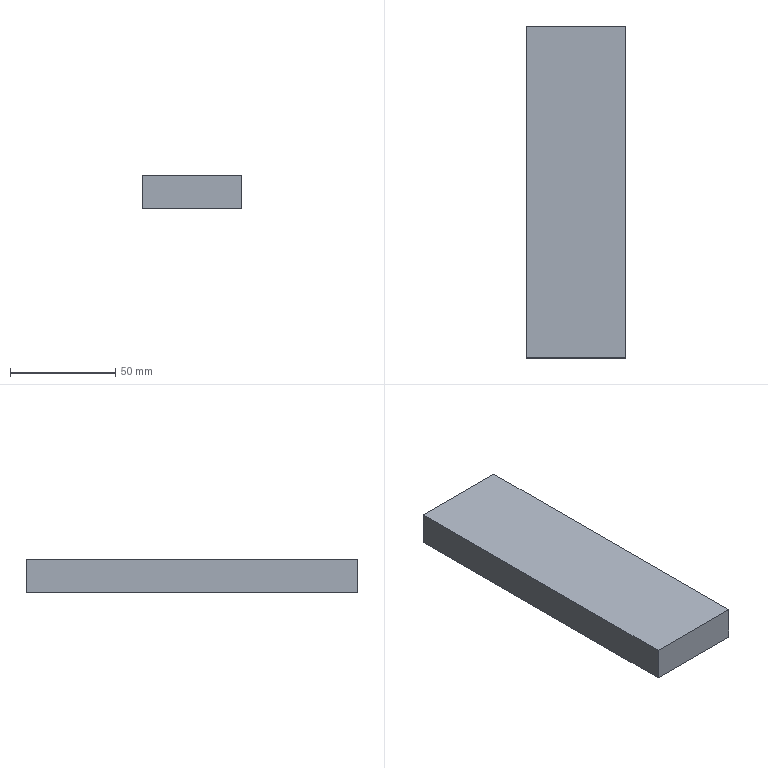Part | STEP file | 04-Square plate | 1 solid | 6 faces | box 47.5 x 158 x 16 mm | volume 120080 mm3 | plane 6
STEP:
#1=CARTESIAN_POINT('',(0.,0.,0.));
#2=DIRECTION('',(0.,0.,1.));
#3=DIRECTION('',(1.,0.,0.));
#4=AXIS2_PLACEMENT_3D('',#1,#2,#3);
#5=CARTESIAN_POINT('',(0.,0.,0.));
#6=VERTEX_POINT('',#5);
#7=CARTESIAN_POINT('',(0.,-158.,0.));
#8=VERTEX_POINT('',#7);
#9=CARTESIAN_POINT('',(0.,0.,0.));
#10=DIRECTION('',(0.,-1.,0.));
#11=VECTOR('',#10,1.);
#12=LINE('',#9,#11);
#13=CARTESIAN_POINT('',(0.,0.,16.));
#14=DIRECTION('',(1.,0.,0.));
#15=DIRECTION('',(0.,1.,0.));
#16=AXIS2_PLACEMENT_3D('',#13,#14,#15);
#17=PLANE('',#16);
#18=CARTESIAN_POINT('',(0.,-16.));
#19=DIRECTION('',(-1.,0.));
#20=VECTOR('',#19,1.);
#21=LINE('',#18,#20);
#22=(GEOMETRIC_REPRESENTATION_CONTEXT(2)PARAMETRIC_REPRESENTATION_CONTEXT()REPRESENTATION_CONTEXT('',''));
#23=DEFINITIONAL_REPRESENTATION('',(#21),#22);
#24=PCURVE('',#17,#23);
#25=CARTESIAN_POINT('',(0.,0.,0.));
#26=DIRECTION('',(0.,0.,1.));
#27=DIRECTION('',(1.,0.,0.));
#28=AXIS2_PLACEMENT_3D('',#25,#26,#27);
#29=PLANE('',#28);
#30=CARTESIAN_POINT('',(0.,0.));
#31=DIRECTION('',(0.,-1.));
#32=VECTOR('',#31,1.);
#33=LINE('',#30,#32);
#34=(GEOMETRIC_REPRESENTATION_CONTEXT(2)PARAMETRIC_REPRESENTATION_CONTEXT()REPRESENTATION_CONTEXT('',''));
#35=DEFINITIONAL_REPRESENTATION('',(#33),#34);
#36=PCURVE('',#29,#35);
#37=SURFACE_CURVE('',#12,(#24,#36),.PCURVE_S1.);
#38=EDGE_CURVE('',#6,#8,#37,.T.);
#39=ORIENTED_EDGE('',*,*,#38,.T.);
#40=CARTESIAN_POINT('',(0.,-158.,16.));
#41=VERTEX_POINT('',#40);
#42=CARTESIAN_POINT('',(0.,-158.,16.));
#43=DIRECTION('',(0.,0.,-1.));
#44=VECTOR('',#43,1.);
#45=LINE('',#42,#44);
#46=CARTESIAN_POINT('',(-158.,0.));
#47=DIRECTION('',(0.,-1.));
#48=VECTOR('',#47,1.);
#49=LINE('',#46,#48);
#50=(GEOMETRIC_REPRESENTATION_CONTEXT(2)PARAMETRIC_REPRESENTATION_CONTEXT()REPRESENTATION_CONTEXT('',''));
#51=DEFINITIONAL_REPRESENTATION('',(#49),#50);
#52=PCURVE('',#17,#51);
#53=CARTESIAN_POINT('',(0.,-158.,16.));
#54=DIRECTION('',(0.,1.,0.));
#55=DIRECTION('',(0.,0.,1.));
#56=AXIS2_PLACEMENT_3D('',#53,#54,#55);
#57=PLANE('',#56);
#58=CARTESIAN_POINT('',(0.,0.));
#59=DIRECTION('',(-1.,0.));
#60=VECTOR('',#59,1.);
#61=LINE('',#58,#60);
#62=(GEOMETRIC_REPRESENTATION_CONTEXT(2)PARAMETRIC_REPRESENTATION_CONTEXT()REPRESENTATION_CONTEXT('',''));
#63=DEFINITIONAL_REPRESENTATION('',(#61),#62);
#64=PCURVE('',#57,#63);
#65=SURFACE_CURVE('',#45,(#52,#64),.PCURVE_S1.);
#66=EDGE_CURVE('',#41,#8,#65,.T.);
#67=ORIENTED_EDGE('',*,*,#66,.F.);
#68=CARTESIAN_POINT('',(0.,0.,16.));
#69=VERTEX_POINT('',#68);
#70=CARTESIAN_POINT('',(0.,0.,16.));
#71=DIRECTION('',(0.,-1.,0.));
#72=VECTOR('',#71,1.);
#73=LINE('',#70,#72);
#74=CARTESIAN_POINT('',(0.,0.));
#75=DIRECTION('',(-1.,0.));
#76=VECTOR('',#75,1.);
#77=LINE('',#74,#76);
#78=(GEOMETRIC_REPRESENTATION_CONTEXT(2)PARAMETRIC_REPRESENTATION_CONTEXT()REPRESENTATION_CONTEXT('',''));
#79=DEFINITIONAL_REPRESENTATION('',(#77),#78);
#80=PCURVE('',#17,#79);
#81=CARTESIAN_POINT('',(0.,0.,16.));
#82=DIRECTION('',(0.,0.,1.));
#83=DIRECTION('',(1.,0.,0.));
#84=AXIS2_PLACEMENT_3D('',#81,#82,#83);
#85=PLANE('',#84);
#86=CARTESIAN_POINT('',(0.,0.));
#87=DIRECTION('',(0.,-1.));
#88=VECTOR('',#87,1.);
#89=LINE('',#86,#88);
#90=(GEOMETRIC_REPRESENTATION_CONTEXT(2)PARAMETRIC_REPRESENTATION_CONTEXT()REPRESENTATION_CONTEXT('',''));
#91=DEFINITIONAL_REPRESENTATION('',(#89),#90);
#92=PCURVE('',#85,#91);
#93=SURFACE_CURVE('',#73,(#80,#92),.PCURVE_S1.);
#94=EDGE_CURVE('',#69,#41,#93,.T.);
#95=ORIENTED_EDGE('',*,*,#94,.F.);
#96=CARTESIAN_POINT('',(0.,0.,16.));
#97=DIRECTION('',(0.,0.,-1.));
#98=VECTOR('',#97,1.);
#99=LINE('',#96,#98);
#100=CARTESIAN_POINT('',(0.,0.));
#101=DIRECTION('',(0.,-1.));
#102=VECTOR('',#101,1.);
#103=LINE('',#100,#102);
#104=(GEOMETRIC_REPRESENTATION_CONTEXT(2)PARAMETRIC_REPRESENTATION_CONTEXT()REPRESENTATION_CONTEXT('',''));
#105=DEFINITIONAL_REPRESENTATION('',(#103),#104);
#106=PCURVE('',#17,#105);
#107=CARTESIAN_POINT('',(0.,0.,16.));
#108=DIRECTION('',(0.,-1.,0.));
#109=DIRECTION('',(0.,0.,-1.));
#110=AXIS2_PLACEMENT_3D('',#107,#108,#109);
#111=PLANE('',#110);
#112=CARTESIAN_POINT('',(0.,0.));
#113=DIRECTION('',(1.,0.));
#114=VECTOR('',#113,1.);
#115=LINE('',#112,#114);
#116=(GEOMETRIC_REPRESENTATION_CONTEXT(2)PARAMETRIC_REPRESENTATION_CONTEXT()REPRESENTATION_CONTEXT('',''));
#117=DEFINITIONAL_REPRESENTATION('',(#115),#116);
#118=PCURVE('',#111,#117);
#119=SURFACE_CURVE('',#99,(#106,#118),.PCURVE_S1.);
#120=EDGE_CURVE('',#69,#6,#119,.T.);
#121=ORIENTED_EDGE('',*,*,#120,.T.);
#122=EDGE_LOOP('',(#39,#67,#95,#121));
#123=FACE_BOUND('',#122,.T.);
#124=ADVANCED_FACE('',(#123),#17,.F.);
#125=CARTESIAN_POINT('',(47.5,-158.,0.));
#126=VERTEX_POINT('',#125);
#127=CARTESIAN_POINT('',(0.,-158.,0.));
#128=DIRECTION('',(1.,0.,0.));
#129=VECTOR('',#128,1.);
#130=LINE('',#127,#129);
#131=CARTESIAN_POINT('',(-16.,0.));
#132=DIRECTION('',(0.,1.));
#133=VECTOR('',#132,1.);
#134=LINE('',#131,#133);
#135=(GEOMETRIC_REPRESENTATION_CONTEXT(2)PARAMETRIC_REPRESENTATION_CONTEXT()REPRESENTATION_CONTEXT('',''));
#136=DEFINITIONAL_REPRESENTATION('',(#134),#135);
#137=PCURVE('',#57,#136);
#138=CARTESIAN_POINT('',(0.,-158.));
#139=DIRECTION('',(1.,0.));
#140=VECTOR('',#139,1.);
#141=LINE('',#138,#140);
#142=(GEOMETRIC_REPRESENTATION_CONTEXT(2)PARAMETRIC_REPRESENTATION_CONTEXT()REPRESENTATION_CONTEXT('',''));
#143=DEFINITIONAL_REPRESENTATION('',(#141),#142);
#144=PCURVE('',#29,#143);
#145=SURFACE_CURVE('',#130,(#137,#144),.PCURVE_S1.);
#146=EDGE_CURVE('',#8,#126,#145,.T.);
#147=ORIENTED_EDGE('',*,*,#146,.T.);
#148=CARTESIAN_POINT('',(47.5,-158.,16.));
#149=VERTEX_POINT('',#148);
#150=CARTESIAN_POINT('',(47.5,-158.,16.));
#151=DIRECTION('',(0.,0.,-1.));
#152=VECTOR('',#151,1.);
#153=LINE('',#150,#152);
#154=CARTESIAN_POINT('',(0.,47.5));
#155=DIRECTION('',(-1.,0.));
#156=VECTOR('',#155,1.);
#157=LINE('',#154,#156);
#158=(GEOMETRIC_REPRESENTATION_CONTEXT(2)PARAMETRIC_REPRESENTATION_CONTEXT()REPRESENTATION_CONTEXT('',''));
#159=DEFINITIONAL_REPRESENTATION('',(#157),#158);
#160=PCURVE('',#57,#159);
#161=CARTESIAN_POINT('',(47.5,0.,16.));
#162=DIRECTION('',(-1.,0.,0.));
#163=DIRECTION('',(0.,-1.,0.));
#164=AXIS2_PLACEMENT_3D('',#161,#162,#163);
#165=PLANE('',#164);
#166=CARTESIAN_POINT('',(158.,0.));
#167=DIRECTION('',(0.,-1.));
#168=VECTOR('',#167,1.);
#169=LINE('',#166,#168);
#170=(GEOMETRIC_REPRESENTATION_CONTEXT(2)PARAMETRIC_REPRESENTATION_CONTEXT()REPRESENTATION_CONTEXT('',''));
#171=DEFINITIONAL_REPRESENTATION('',(#169),#170);
#172=PCURVE('',#165,#171);
#173=SURFACE_CURVE('',#153,(#160,#172),.PCURVE_S1.);
#174=EDGE_CURVE('',#149,#126,#173,.T.);
#175=ORIENTED_EDGE('',*,*,#174,.F.);
#176=CARTESIAN_POINT('',(0.,-158.,16.));
#177=DIRECTION('',(1.,0.,0.));
#178=VECTOR('',#177,1.);
#179=LINE('',#176,#178);
#180=CARTESIAN_POINT('',(0.,0.));
#181=DIRECTION('',(0.,1.));
#182=VECTOR('',#181,1.);
#183=LINE('',#180,#182);
#184=(GEOMETRIC_REPRESENTATION_CONTEXT(2)PARAMETRIC_REPRESENTATION_CONTEXT()REPRESENTATION_CONTEXT('',''));
#185=DEFINITIONAL_REPRESENTATION('',(#183),#184);
#186=PCURVE('',#57,#185);
#187=CARTESIAN_POINT('',(0.,-158.));
#188=DIRECTION('',(1.,0.));
#189=VECTOR('',#188,1.);
#190=LINE('',#187,#189);
#191=(GEOMETRIC_REPRESENTATION_CONTEXT(2)PARAMETRIC_REPRESENTATION_CONTEXT()REPRESENTATION_CONTEXT('',''));
#192=DEFINITIONAL_REPRESENTATION('',(#190),#191);
#193=PCURVE('',#85,#192);
#194=SURFACE_CURVE('',#179,(#186,#193),.PCURVE_S1.);
#195=EDGE_CURVE('',#41,#149,#194,.T.);
#196=ORIENTED_EDGE('',*,*,#195,.F.);
#197=ORIENTED_EDGE('',*,*,#66,.T.);
#198=EDGE_LOOP('',(#147,#175,#196,#197));
#199=FACE_BOUND('',#198,.T.);
#200=ADVANCED_FACE('',(#199),#57,.F.);
#201=CARTESIAN_POINT('',(47.5,0.,0.));
#202=VERTEX_POINT('',#201);
#203=CARTESIAN_POINT('',(47.5,0.,0.));
#204=DIRECTION('',(0.,1.,0.));
#205=VECTOR('',#204,1.);
#206=LINE('',#203,#205);
#207=CARTESIAN_POINT('',(0.,-16.));
#208=DIRECTION('',(-1.,0.));
#209=VECTOR('',#208,1.);
#210=LINE('',#207,#209);
#211=(GEOMETRIC_REPRESENTATION_CONTEXT(2)PARAMETRIC_REPRESENTATION_CONTEXT()REPRESENTATION_CONTEXT('',''));
#212=DEFINITIONAL_REPRESENTATION('',(#210),#211);
#213=PCURVE('',#165,#212);
#214=CARTESIAN_POINT('',(47.5,0.));
#215=DIRECTION('',(0.,1.));
#216=VECTOR('',#215,1.);
#217=LINE('',#214,#216);
#218=(GEOMETRIC_REPRESENTATION_CONTEXT(2)PARAMETRIC_REPRESENTATION_CONTEXT()REPRESENTATION_CONTEXT('',''));
#219=DEFINITIONAL_REPRESENTATION('',(#217),#218);
#220=PCURVE('',#29,#219);
#221=SURFACE_CURVE('',#206,(#213,#220),.PCURVE_S1.);
#222=EDGE_CURVE('',#126,#202,#221,.T.);
#223=ORIENTED_EDGE('',*,*,#222,.T.);
#224=CARTESIAN_POINT('',(47.5,0.,16.));
#225=VERTEX_POINT('',#224);
#226=CARTESIAN_POINT('',(47.5,0.,16.));
#227=DIRECTION('',(0.,0.,-1.));
#228=VECTOR('',#227,1.);
#229=LINE('',#226,#228);
#230=CARTESIAN_POINT('',(0.,0.));
#231=DIRECTION('',(0.,-1.));
#232=VECTOR('',#231,1.);
#233=LINE('',#230,#232);
#234=(GEOMETRIC_REPRESENTATION_CONTEXT(2)PARAMETRIC_REPRESENTATION_CONTEXT()REPRESENTATION_CONTEXT('',''));
#235=DEFINITIONAL_REPRESENTATION('',(#233),#234);
#236=PCURVE('',#165,#235);
#237=CARTESIAN_POINT('',(0.,47.5));
#238=DIRECTION('',(1.,0.));
#239=VECTOR('',#238,1.);
#240=LINE('',#237,#239);
#241=(GEOMETRIC_REPRESENTATION_CONTEXT(2)PARAMETRIC_REPRESENTATION_CONTEXT()REPRESENTATION_CONTEXT('',''));
#242=DEFINITIONAL_REPRESENTATION('',(#240),#241);
#243=PCURVE('',#111,#242);
#244=SURFACE_CURVE('',#229,(#236,#243),.PCURVE_S1.);
#245=EDGE_CURVE('',#225,#202,#244,.T.);
#246=ORIENTED_EDGE('',*,*,#245,.F.);
#247=CARTESIAN_POINT('',(47.5,0.,16.));
#248=DIRECTION('',(0.,1.,0.));
#249=VECTOR('',#248,1.);
#250=LINE('',#247,#249);
#251=CARTESIAN_POINT('',(0.,0.));
#252=DIRECTION('',(-1.,0.));
#253=VECTOR('',#252,1.);
#254=LINE('',#251,#253);
#255=(GEOMETRIC_REPRESENTATION_CONTEXT(2)PARAMETRIC_REPRESENTATION_CONTEXT()REPRESENTATION_CONTEXT('',''));
#256=DEFINITIONAL_REPRESENTATION('',(#254),#255);
#257=PCURVE('',#165,#256);
#258=CARTESIAN_POINT('',(47.5,0.));
#259=DIRECTION('',(0.,1.));
#260=VECTOR('',#259,1.);
#261=LINE('',#258,#260);
#262=(GEOMETRIC_REPRESENTATION_CONTEXT(2)PARAMETRIC_REPRESENTATION_CONTEXT()REPRESENTATION_CONTEXT('',''));
#263=DEFINITIONAL_REPRESENTATION('',(#261),#262);
#264=PCURVE('',#85,#263);
#265=SURFACE_CURVE('',#250,(#257,#264),.PCURVE_S1.);
#266=EDGE_CURVE('',#149,#225,#265,.T.);
#267=ORIENTED_EDGE('',*,*,#266,.F.);
#268=ORIENTED_EDGE('',*,*,#174,.T.);
#269=EDGE_LOOP('',(#223,#246,#267,#268));
#270=FACE_BOUND('',#269,.T.);
#271=ADVANCED_FACE('',(#270),#165,.F.);
#272=CARTESIAN_POINT('',(0.,0.,0.));
#273=DIRECTION('',(-1.,0.,0.));
#274=VECTOR('',#273,1.);
#275=LINE('',#272,#274);
#276=CARTESIAN_POINT('',(16.,0.));
#277=DIRECTION('',(0.,-1.));
#278=VECTOR('',#277,1.);
#279=LINE('',#276,#278);
#280=(GEOMETRIC_REPRESENTATION_CONTEXT(2)PARAMETRIC_REPRESENTATION_CONTEXT()REPRESENTATION_CONTEXT('',''));
#281=DEFINITIONAL_REPRESENTATION('',(#279),#280);
#282=PCURVE('',#111,#281);
#283=CARTESIAN_POINT('',(0.,0.));
#284=DIRECTION('',(-1.,0.));
#285=VECTOR('',#284,1.);
#286=LINE('',#283,#285);
#287=(GEOMETRIC_REPRESENTATION_CONTEXT(2)PARAMETRIC_REPRESENTATION_CONTEXT()REPRESENTATION_CONTEXT('',''));
#288=DEFINITIONAL_REPRESENTATION('',(#286),#287);
#289=PCURVE('',#29,#288);
#290=SURFACE_CURVE('',#275,(#282,#289),.PCURVE_S1.);
#291=EDGE_CURVE('',#202,#6,#290,.T.);
#292=ORIENTED_EDGE('',*,*,#291,.T.);
#293=ORIENTED_EDGE('',*,*,#120,.F.);
#294=CARTESIAN_POINT('',(0.,0.,16.));
#295=DIRECTION('',(-1.,0.,0.));
#296=VECTOR('',#295,1.);
#297=LINE('',#294,#296);
#298=CARTESIAN_POINT('',(0.,0.));
#299=DIRECTION('',(0.,-1.));
#300=VECTOR('',#299,1.);
#301=LINE('',#298,#300);
#302=(GEOMETRIC_REPRESENTATION_CONTEXT(2)PARAMETRIC_REPRESENTATION_CONTEXT()REPRESENTATION_CONTEXT('',''));
#303=DEFINITIONAL_REPRESENTATION('',(#301),#302);
#304=PCURVE('',#111,#303);
#305=CARTESIAN_POINT('',(0.,0.));
#306=DIRECTION('',(-1.,0.));
#307=VECTOR('',#306,1.);
#308=LINE('',#305,#307);
#309=(GEOMETRIC_REPRESENTATION_CONTEXT(2)PARAMETRIC_REPRESENTATION_CONTEXT()REPRESENTATION_CONTEXT('',''));
#310=DEFINITIONAL_REPRESENTATION('',(#308),#309);
#311=PCURVE('',#85,#310);
#312=SURFACE_CURVE('',#297,(#304,#311),.PCURVE_S1.);
#313=EDGE_CURVE('',#225,#69,#312,.T.);
#314=ORIENTED_EDGE('',*,*,#313,.F.);
#315=ORIENTED_EDGE('',*,*,#245,.T.);
#316=EDGE_LOOP('',(#292,#293,#314,#315));
#317=FACE_BOUND('',#316,.T.);
#318=ADVANCED_FACE('',(#317),#111,.F.);
#319=ORIENTED_EDGE('',*,*,#94,.T.);
#320=ORIENTED_EDGE('',*,*,#195,.T.);
#321=ORIENTED_EDGE('',*,*,#266,.T.);
#322=ORIENTED_EDGE('',*,*,#313,.T.);
#323=EDGE_LOOP('',(#319,#320,#321,#322));
#324=FACE_BOUND('',#323,.T.);
#325=ADVANCED_FACE('',(#324),#85,.T.);
#326=ORIENTED_EDGE('',*,*,#38,.F.);
#327=ORIENTED_EDGE('',*,*,#291,.F.);
#328=ORIENTED_EDGE('',*,*,#222,.F.);
#329=ORIENTED_EDGE('',*,*,#146,.F.);
#330=EDGE_LOOP('',(#326,#327,#328,#329));
#331=FACE_BOUND('',#330,.T.);
#332=ADVANCED_FACE('',(#331),#29,.F.);
#333=CLOSED_SHELL('',(#124,#200,#271,#318,#325,#332));
#334=MANIFOLD_SOLID_BREP('',#333);
#335=(LENGTH_UNIT()NAMED_UNIT(*)SI_UNIT(.MILLI.,.METRE.));
#336=UNCERTAINTY_MEASURE_WITH_UNIT(LENGTH_MEASURE(0.0000001),#335,'','');
#337=(NAMED_UNIT(*)PLANE_ANGLE_UNIT()SI_UNIT($,.RADIAN.));
#338=(NAMED_UNIT(*)SI_UNIT($,.STERADIAN.)SOLID_ANGLE_UNIT());
#339=(GEOMETRIC_REPRESENTATION_CONTEXT(3)GLOBAL_UNCERTAINTY_ASSIGNED_CONTEXT((#336))GLOBAL_UNIT_ASSIGNED_CONTEXT((#335,#337,#338))REPRESENTATION_CONTEXT('',''));
#340=ADVANCED_BREP_SHAPE_REPRESENTATION('',(#4,#334),#339);